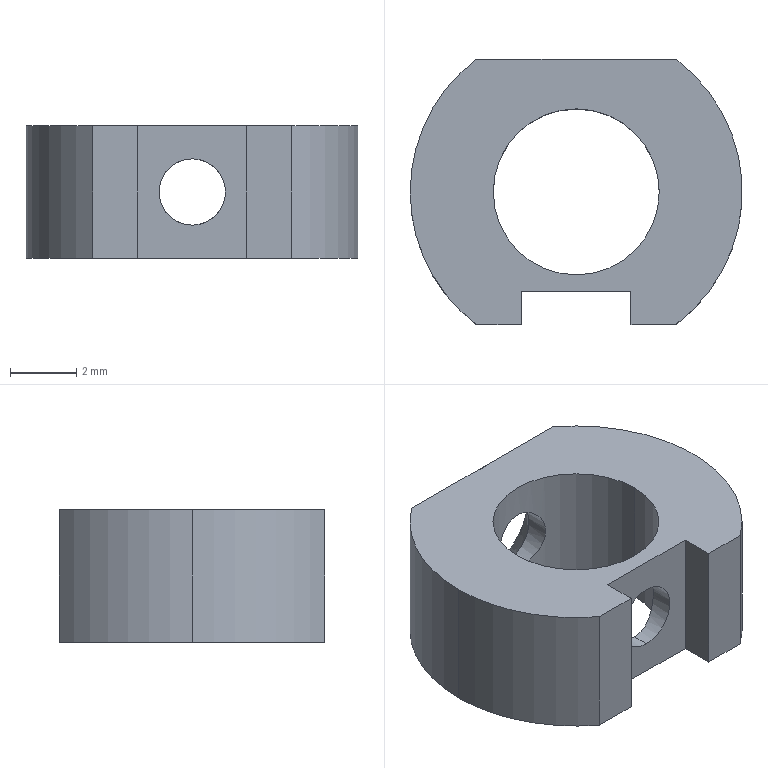Part | SolidWorks | features BaseBody 1 | 1 solid | 20 faces | box 10 x 8 x 4 mm | volume 178.926 mm3 | cylinder 9 | plane 9 | cone 2 | commonest cylinder face diameters 2 x4 10 x3 5 x2
STEP:
#1=CARTESIAN_POINT('',(-5.,0.,4.5));
#2=VERTEX_POINT('',#1);
#3=CARTESIAN_POINT('',(-3.,-4.,4.5));
#4=VERTEX_POINT('',#3);
#5=CARTESIAN_POINT('',(0.,0.,4.5));
#6=DIRECTION('',(0.,0.,1.));
#7=DIRECTION('',(-1.,0.,0.));
#8=AXIS2_PLACEMENT_3D('',#5,#6,#7);
#9=CIRCLE('',#8,5.);
#10=EDGE_CURVE('',#2,#4,#9,.T.);
#11=ORIENTED_EDGE('',*,*,#10,.F.);
#12=CARTESIAN_POINT('',(-5.,0.,0.5));
#13=VERTEX_POINT('',#12);
#14=CARTESIAN_POINT('',(-5.,0.,5.));
#15=DIRECTION('',(0.,0.,-1.));
#16=VECTOR('',#15,1000.);
#17=LINE('',#14,#16);
#18=EDGE_CURVE('',#2,#13,#17,.T.);
#19=ORIENTED_EDGE('',*,*,#18,.T.);
#20=CARTESIAN_POINT('',(-3.,-4.,0.5));
#21=VERTEX_POINT('',#20);
#22=CARTESIAN_POINT('',(0.,0.,0.5));
#23=DIRECTION('',(0.,0.,1.));
#24=DIRECTION('',(-1.,0.,0.));
#25=AXIS2_PLACEMENT_3D('',#22,#23,#24);
#26=CIRCLE('',#25,5.);
#27=EDGE_CURVE('',#13,#21,#26,.T.);
#28=ORIENTED_EDGE('',*,*,#27,.T.);
#29=CARTESIAN_POINT('',(-3.,-4.,5.));
#30=DIRECTION('',(0.,0.,1.));
#31=VECTOR('',#30,1000.);
#32=LINE('',#29,#31);
#33=EDGE_CURVE('',#21,#4,#32,.T.);
#34=ORIENTED_EDGE('',*,*,#33,.T.);
#35=EDGE_LOOP('',(#11,#19,#28,#34));
#36=FACE_OUTER_BOUND('',#35,.T.);
#37=CARTESIAN_POINT('',(0.,0.,5.));
#38=DIRECTION('',(0.,0.,-1.));
#39=DIRECTION('',(-1.,0.,0.));
#40=AXIS2_PLACEMENT_3D('',#37,#38,#39);
#41=CYLINDRICAL_SURFACE('',#40,5.);
#42=ADVANCED_FACE('',(#36),#41,.T.);
#43=CARTESIAN_POINT('',(0.,-2.5,3.5));
#44=VERTEX_POINT('',#43);
#45=CARTESIAN_POINT('',(0.,-2.5,1.5));
#46=VERTEX_POINT('',#45);
#47=CARTESIAN_POINT('',(0.,-2.5,3.5));
#48=CARTESIAN_POINT('',(0.1336,-2.5,3.5));
#49=CARTESIAN_POINT('',(0.2646,-2.489,3.473));
#50=CARTESIAN_POINT('',(0.5062,-2.451,3.372));
#51=CARTESIAN_POINT('',(0.6161,-2.425,3.298));
#52=CARTESIAN_POINT('',(0.7985,-2.371,3.116));
#53=CARTESIAN_POINT('',(0.8726,-2.343,3.006));
#54=CARTESIAN_POINT('',(0.9728,-2.304,2.766));
#55=CARTESIAN_POINT('',(0.9998,-2.291,2.633));
#56=CARTESIAN_POINT('',(1.,-2.291,2.369));
#57=CARTESIAN_POINT('',(0.9739,-2.303,2.238));
#58=CARTESIAN_POINT('',(0.8725,-2.343,1.994));
#59=CARTESIAN_POINT('',(0.799,-2.371,1.885));
#60=CARTESIAN_POINT('',(0.6162,-2.425,1.702));
#61=CARTESIAN_POINT('',(0.506,-2.451,1.628));
#62=CARTESIAN_POINT('',(0.2658,-2.489,1.527));
#63=CARTESIAN_POINT('',(0.1336,-2.5,1.5));
#64=CARTESIAN_POINT('',(0.,-2.5,1.5));
#65=B_SPLINE_CURVE_WITH_KNOTS('',3,(#47,#48,#49,#50,#51,#52,#53,#54,#55,#56,#57,#58,#59,#60,#61,#62,#63,#64),.UNSPECIFIED.,.F.,.F.,(4,2,2,2,2,2,2,2,4),(0.,0.0003948,0.0007896,0.001184,0.001579,0.001974,0.002369,0.002764,0.003158),.UNSPECIFIED.);
#66=EDGE_CURVE('',#44,#46,#65,.T.);
#67=ORIENTED_EDGE('',*,*,#66,.F.);
#68=CARTESIAN_POINT('',(0.,-2.5,1.5));
#69=CARTESIAN_POINT('',(-0.1336,-2.5,1.5));
#70=CARTESIAN_POINT('',(-0.2646,-2.489,1.527));
#71=CARTESIAN_POINT('',(-0.5062,-2.451,1.628));
#72=CARTESIAN_POINT('',(-0.6161,-2.425,1.702));
#73=CARTESIAN_POINT('',(-0.7985,-2.371,1.884));
#74=CARTESIAN_POINT('',(-0.8726,-2.343,1.994));
#75=CARTESIAN_POINT('',(-0.9728,-2.304,2.234));
#76=CARTESIAN_POINT('',(-0.9998,-2.291,2.367));
#77=CARTESIAN_POINT('',(-1.,-2.291,2.631));
#78=CARTESIAN_POINT('',(-0.9739,-2.303,2.762));
#79=CARTESIAN_POINT('',(-0.8725,-2.343,3.006));
#80=CARTESIAN_POINT('',(-0.799,-2.371,3.115));
#81=CARTESIAN_POINT('',(-0.6162,-2.425,3.298));
#82=CARTESIAN_POINT('',(-0.506,-2.451,3.372));
#83=CARTESIAN_POINT('',(-0.2658,-2.489,3.473));
#84=CARTESIAN_POINT('',(-0.1336,-2.5,3.5));
#85=CARTESIAN_POINT('',(0.,-2.5,3.5));
#86=B_SPLINE_CURVE_WITH_KNOTS('',3,(#68,#69,#70,#71,#72,#73,#74,#75,#76,#77,#78,#79,#80,#81,#82,#83,#84,#85),.UNSPECIFIED.,.F.,.F.,(4,2,2,2,2,2,2,2,4),(0.003158,0.003553,0.003948,0.004343,0.004737,0.005132,0.005527,0.005921,0.006316),.UNSPECIFIED.);
#87=EDGE_CURVE('',#46,#44,#86,.T.);
#88=ORIENTED_EDGE('',*,*,#87,.F.);
#89=EDGE_LOOP('',(#67,#88));
#90=FACE_BOUND('',#89,.T.);
#91=CARTESIAN_POINT('',(2.5,0.,4.5));
#92=VERTEX_POINT('',#91);
#93=CARTESIAN_POINT('',(-2.5,0.,4.5));
#94=VERTEX_POINT('',#93);
#95=CARTESIAN_POINT('',(0.,0.,4.5));
#96=DIRECTION('',(0.,0.,-1.));
#97=DIRECTION('',(-1.,0.,0.));
#98=AXIS2_PLACEMENT_3D('',#95,#96,#97);
#99=CIRCLE('',#98,2.5);
#100=EDGE_CURVE('',#92,#94,#99,.T.);
#101=ORIENTED_EDGE('',*,*,#100,.F.);
#102=CARTESIAN_POINT('',(2.5,0.,0.5));
#103=VERTEX_POINT('',#102);
#104=CARTESIAN_POINT('',(2.5,0.,5.));
#105=DIRECTION('',(0.,0.,-1.));
#106=VECTOR('',#105,1000.);
#107=LINE('',#104,#106);
#108=EDGE_CURVE('',#92,#103,#107,.T.);
#109=ORIENTED_EDGE('',*,*,#108,.T.);
#110=CARTESIAN_POINT('',(-2.5,0.,0.5));
#111=VERTEX_POINT('',#110);
#112=CARTESIAN_POINT('',(0.,0.,0.5));
#113=DIRECTION('',(0.,0.,1.));
#114=DIRECTION('',(-1.,0.,0.));
#115=AXIS2_PLACEMENT_3D('',#112,#113,#114);
#116=CIRCLE('',#115,2.5);
#117=EDGE_CURVE('',#111,#103,#116,.T.);
#118=ORIENTED_EDGE('',*,*,#117,.F.);
#119=CARTESIAN_POINT('',(-2.5,0.,5.));
#120=DIRECTION('',(0.,0.,-1.));
#121=VECTOR('',#120,1000.);
#122=LINE('',#119,#121);
#123=EDGE_CURVE('',#94,#111,#122,.T.);
#124=ORIENTED_EDGE('',*,*,#123,.F.);
#125=EDGE_LOOP('',(#101,#109,#118,#124));
#126=FACE_OUTER_BOUND('',#125,.T.);
#127=CARTESIAN_POINT('',(0.,0.,5.));
#128=DIRECTION('',(0.,0.,-1.));
#129=DIRECTION('',(-1.,0.,0.));
#130=AXIS2_PLACEMENT_3D('',#127,#128,#129);
#131=CYLINDRICAL_SURFACE('',#130,2.5);
#132=ADVANCED_FACE('',(#90,#126),#131,.F.);
#133=CARTESIAN_POINT('',(0.,-3.,3.5));
#134=VERTEX_POINT('',#133);
#135=CARTESIAN_POINT('',(0.,-3.,1.5));
#136=VERTEX_POINT('',#135);
#137=CARTESIAN_POINT('',(0.,-3.,2.5));
#138=DIRECTION('',(0.,-1.,0.));
#139=DIRECTION('',(0.,0.,1.));
#140=AXIS2_PLACEMENT_3D('',#137,#138,#139);
#141=CIRCLE('',#140,1.);
#142=EDGE_CURVE('',#134,#136,#141,.T.);
#143=ORIENTED_EDGE('',*,*,#142,.T.);
#144=CARTESIAN_POINT('',(0.,-6.,1.5));
#145=DIRECTION('',(0.,1.,0.));
#146=VECTOR('',#145,1000.);
#147=LINE('',#144,#146);
#148=EDGE_CURVE('',#136,#46,#147,.T.);
#149=ORIENTED_EDGE('',*,*,#148,.T.);
#150=ORIENTED_EDGE('',*,*,#87,.T.);
#151=CARTESIAN_POINT('',(0.,-6.,3.5));
#152=DIRECTION('',(0.,1.,0.));
#153=VECTOR('',#152,1000.);
#154=LINE('',#151,#153);
#155=EDGE_CURVE('',#134,#44,#154,.T.);
#156=ORIENTED_EDGE('',*,*,#155,.F.);
#157=EDGE_LOOP('',(#143,#149,#150,#156));
#158=FACE_OUTER_BOUND('',#157,.T.);
#159=CARTESIAN_POINT('',(0.,-6.,2.5));
#160=DIRECTION('',(0.,1.,0.));
#161=DIRECTION('',(0.,0.,1.));
#162=AXIS2_PLACEMENT_3D('',#159,#160,#161);
#163=CYLINDRICAL_SURFACE('',#162,1.);
#164=ADVANCED_FACE('',(#158),#163,.F.);
#165=CARTESIAN_POINT('',(0.,3.,1.5));
#166=VERTEX_POINT('',#165);
#167=CARTESIAN_POINT('',(0.,3.,3.5));
#168=VERTEX_POINT('',#167);
#169=CARTESIAN_POINT('',(0.,3.,2.5));
#170=DIRECTION('',(0.,1.,0.));
#171=DIRECTION('',(0.,0.,1.));
#172=AXIS2_PLACEMENT_3D('',#169,#170,#171);
#173=CIRCLE('',#172,1.);
#174=EDGE_CURVE('',#166,#168,#173,.T.);
#175=ORIENTED_EDGE('',*,*,#174,.F.);
#176=CARTESIAN_POINT('',(0.,4.,0.5));
#177=VERTEX_POINT('',#176);
#178=CARTESIAN_POINT('',(0.,4.,0.5));
#179=DIRECTION('',(0.,0.7071,-0.7071));
#180=VECTOR('',#179,1000.);
#181=LINE('',#178,#180);
#182=EDGE_CURVE('',#166,#177,#181,.T.);
#183=ORIENTED_EDGE('',*,*,#182,.T.);
#184=CARTESIAN_POINT('',(0.,4.,4.5));
#185=VERTEX_POINT('',#184);
#186=CARTESIAN_POINT('',(0.,4.,2.5));
#187=DIRECTION('',(0.,1.,0.));
#188=DIRECTION('',(0.,0.,1.));
#189=AXIS2_PLACEMENT_3D('',#186,#187,#188);
#190=CIRCLE('',#189,2.);
#191=EDGE_CURVE('',#177,#185,#190,.T.);
#192=ORIENTED_EDGE('',*,*,#191,.T.);
#193=CARTESIAN_POINT('',(0.,4.,4.5));
#194=DIRECTION('',(0.,0.7071,0.7071));
#195=VECTOR('',#194,1000.);
#196=LINE('',#193,#195);
#197=EDGE_CURVE('',#168,#185,#196,.T.);
#198=ORIENTED_EDGE('',*,*,#197,.F.);
#199=EDGE_LOOP('',(#175,#183,#192,#198));
#200=FACE_OUTER_BOUND('',#199,.T.);
#201=CARTESIAN_POINT('',(0.,4.,2.5));
#202=DIRECTION('',(0.,1.,0.));
#203=DIRECTION('',(0.,0.,1.));
#204=AXIS2_PLACEMENT_3D('',#201,#202,#203);
#205=CONICAL_SURFACE('',#204,2.,0.7854);
#206=ADVANCED_FACE('',(#200),#205,.F.);
#207=CARTESIAN_POINT('',(0.,2.5,3.5));
#208=VERTEX_POINT('',#207);
#209=CARTESIAN_POINT('',(0.,2.5,1.5));
#210=VERTEX_POINT('',#209);
#211=CARTESIAN_POINT('',(0.,2.5,3.5));
#212=CARTESIAN_POINT('',(-0.1336,2.5,3.5));
#213=CARTESIAN_POINT('',(-0.2646,2.489,3.473));
#214=CARTESIAN_POINT('',(-0.5062,2.451,3.372));
#215=CARTESIAN_POINT('',(-0.6161,2.425,3.298));
#216=CARTESIAN_POINT('',(-0.7985,2.371,3.116));
#217=CARTESIAN_POINT('',(-0.8726,2.343,3.006));
#218=CARTESIAN_POINT('',(-0.9728,2.304,2.766));
#219=CARTESIAN_POINT('',(-0.9998,2.291,2.633));
#220=CARTESIAN_POINT('',(-1.,2.291,2.369));
#221=CARTESIAN_POINT('',(-0.9739,2.303,2.238));
#222=CARTESIAN_POINT('',(-0.8725,2.343,1.994));
#223=CARTESIAN_POINT('',(-0.799,2.371,1.885));
#224=CARTESIAN_POINT('',(-0.6162,2.425,1.702));
#225=CARTESIAN_POINT('',(-0.506,2.451,1.628));
#226=CARTESIAN_POINT('',(-0.2658,2.489,1.527));
#227=CARTESIAN_POINT('',(-0.1336,2.5,1.5));
#228=CARTESIAN_POINT('',(0.,2.5,1.5));
#229=B_SPLINE_CURVE_WITH_KNOTS('',3,(#211,#212,#213,#214,#215,#216,#217,#218,#219,#220,#221,#222,#223,#224,#225,#226,#227,#228),.UNSPECIFIED.,.F.,.F.,(4,2,2,2,2,2,2,2,4),(0.,0.0003948,0.0007896,0.001184,0.001579,0.001974,0.002369,0.002764,0.003158),.UNSPECIFIED.);
#230=EDGE_CURVE('',#208,#210,#229,.T.);
#231=ORIENTED_EDGE('',*,*,#230,.T.);
#232=CARTESIAN_POINT('',(0.,-6.,1.5));
#233=DIRECTION('',(0.,1.,0.));
#234=VECTOR('',#233,1000.);
#235=LINE('',#232,#234);
#236=EDGE_CURVE('',#210,#166,#235,.T.);
#237=ORIENTED_EDGE('',*,*,#236,.T.);
#238=ORIENTED_EDGE('',*,*,#174,.T.);
#239=CARTESIAN_POINT('',(0.,-6.,3.5));
#240=DIRECTION('',(0.,1.,0.));
#241=VECTOR('',#240,1000.);
#242=LINE('',#239,#241);
#243=EDGE_CURVE('',#208,#168,#242,.T.);
#244=ORIENTED_EDGE('',*,*,#243,.F.);
#245=EDGE_LOOP('',(#231,#237,#238,#244));
#246=FACE_OUTER_BOUND('',#245,.T.);
#247=CARTESIAN_POINT('',(0.,-6.,2.5));
#248=DIRECTION('',(0.,1.,0.));
#249=DIRECTION('',(0.,0.,1.));
#250=AXIS2_PLACEMENT_3D('',#247,#248,#249);
#251=CYLINDRICAL_SURFACE('',#250,1.);
#252=ADVANCED_FACE('',(#246),#251,.F.);
#253=CARTESIAN_POINT('',(-1.65,-3.,4.5));
#254=VERTEX_POINT('',#253);
#255=CARTESIAN_POINT('',(1.65,-3.,4.5));
#256=VERTEX_POINT('',#255);
#257=CARTESIAN_POINT('',(0.,-3.,4.5));
#258=DIRECTION('',(1.,0.,0.));
#259=VECTOR('',#258,1000.);
#260=LINE('',#257,#259);
#261=EDGE_CURVE('',#254,#256,#260,.T.);
#262=ORIENTED_EDGE('',*,*,#261,.T.);
#263=CARTESIAN_POINT('',(1.65,-4.,4.5));
#264=VERTEX_POINT('',#263);
#265=CARTESIAN_POINT('',(1.65,-3.,4.5));
#266=DIRECTION('',(0.,-1.,0.));
#267=VECTOR('',#266,1000.);
#268=LINE('',#265,#267);
#269=EDGE_CURVE('',#256,#264,#268,.T.);
#270=ORIENTED_EDGE('',*,*,#269,.T.);
#271=CARTESIAN_POINT('',(3.,-4.,4.5));
#272=VERTEX_POINT('',#271);
#273=CARTESIAN_POINT('',(6.418,-4.,4.5));
#274=DIRECTION('',(1.,0.,0.));
#275=VECTOR('',#274,1000.);
#276=LINE('',#273,#275);
#277=EDGE_CURVE('',#264,#272,#276,.T.);
#278=ORIENTED_EDGE('',*,*,#277,.T.);
#279=CARTESIAN_POINT('',(3.,4.,4.5));
#280=VERTEX_POINT('',#279);
#281=CARTESIAN_POINT('',(0.,0.,4.5));
#282=DIRECTION('',(0.,0.,1.));
#283=DIRECTION('',(-1.,0.,0.));
#284=AXIS2_PLACEMENT_3D('',#281,#282,#283);
#285=CIRCLE('',#284,5.);
#286=EDGE_CURVE('',#272,#280,#285,.T.);
#287=ORIENTED_EDGE('',*,*,#286,.T.);
#288=CARTESIAN_POINT('',(0.,4.,4.5));
#289=DIRECTION('',(-1.,0.,0.));
#290=VECTOR('',#289,1000.);
#291=LINE('',#288,#290);
#292=EDGE_CURVE('',#280,#185,#291,.T.);
#293=ORIENTED_EDGE('',*,*,#292,.T.);
#294=CARTESIAN_POINT('',(-3.,4.,4.5));
#295=VERTEX_POINT('',#294);
#296=CARTESIAN_POINT('',(0.,4.,4.5));
#297=DIRECTION('',(-1.,0.,0.));
#298=VECTOR('',#297,1000.);
#299=LINE('',#296,#298);
#300=EDGE_CURVE('',#185,#295,#299,.T.);
#301=ORIENTED_EDGE('',*,*,#300,.T.);
#302=CARTESIAN_POINT('',(0.,0.,4.5));
#303=DIRECTION('',(0.,0.,1.));
#304=DIRECTION('',(-1.,0.,0.));
#305=AXIS2_PLACEMENT_3D('',#302,#303,#304);
#306=CIRCLE('',#305,5.);
#307=EDGE_CURVE('',#295,#2,#306,.T.);
#308=ORIENTED_EDGE('',*,*,#307,.T.);
#309=ORIENTED_EDGE('',*,*,#10,.T.);
#310=CARTESIAN_POINT('',(-1.65,-4.,4.5));
#311=VERTEX_POINT('',#310);
#312=CARTESIAN_POINT('',(6.418,-4.,4.5));
#313=DIRECTION('',(1.,0.,0.));
#314=VECTOR('',#313,1000.);
#315=LINE('',#312,#314);
#316=EDGE_CURVE('',#4,#311,#315,.T.);
#317=ORIENTED_EDGE('',*,*,#316,.T.);
#318=CARTESIAN_POINT('',(-1.65,-3.,4.5));
#319=DIRECTION('',(0.,1.,0.));
#320=VECTOR('',#319,1000.);
#321=LINE('',#318,#320);
#322=EDGE_CURVE('',#311,#254,#321,.T.);
#323=ORIENTED_EDGE('',*,*,#322,.T.);
#324=EDGE_LOOP('',(#262,#270,#278,#287,#293,#301,#308,#309,#317,#323));
#325=FACE_OUTER_BOUND('',#324,.T.);
#326=CARTESIAN_POINT('',(0.,0.,4.5));
#327=DIRECTION('',(0.,0.,-1.));
#328=DIRECTION('',(-1.,0.,0.));
#329=AXIS2_PLACEMENT_3D('',#326,#327,#328);
#330=CIRCLE('',#329,2.5);
#331=EDGE_CURVE('',#94,#92,#330,.T.);
#332=ORIENTED_EDGE('',*,*,#331,.T.);
#333=ORIENTED_EDGE('',*,*,#100,.T.);
#334=EDGE_LOOP('',(#332,#333));
#335=FACE_BOUND('',#334,.T.);
#336=CARTESIAN_POINT('',(0.,0.,4.5));
#337=DIRECTION('',(0.,0.,1.));
#338=DIRECTION('',(1.,0.,0.));
#339=AXIS2_PLACEMENT_3D('',#336,#337,#338);
#340=PLANE('',#339);
#341=ADVANCED_FACE('',(#325,#335),#340,.T.);
#342=CARTESIAN_POINT('',(1.65,-3.,0.5));
#343=VERTEX_POINT('',#342);
#344=CARTESIAN_POINT('',(1.65,-3.,0.));
#345=DIRECTION('',(0.,0.,-1.));
#346=VECTOR('',#345,1000.);
#347=LINE('',#344,#346);
#348=EDGE_CURVE('',#256,#343,#347,.T.);
#349=ORIENTED_EDGE('',*,*,#348,.F.);
#350=ORIENTED_EDGE('',*,*,#261,.F.);
#351=CARTESIAN_POINT('',(-1.65,-3.,0.5));
#352=VERTEX_POINT('',#351);
#353=CARTESIAN_POINT('',(-1.65,-3.,0.));
#354=DIRECTION('',(0.,0.,1.));
#355=VECTOR('',#354,1000.);
#356=LINE('',#353,#355);
#357=EDGE_CURVE('',#352,#254,#356,.T.);
#358=ORIENTED_EDGE('',*,*,#357,.F.);
#359=CARTESIAN_POINT('',(0.,-3.,0.5));
#360=DIRECTION('',(-1.,0.,0.));
#361=VECTOR('',#360,1000.);
#362=LINE('',#359,#361);
#363=EDGE_CURVE('',#343,#352,#362,.T.);
#364=ORIENTED_EDGE('',*,*,#363,.F.);
#365=EDGE_LOOP('',(#349,#350,#358,#364));
#366=FACE_OUTER_BOUND('',#365,.T.);
#367=ORIENTED_EDGE('',*,*,#142,.F.);
#368=CARTESIAN_POINT('',(0.,-3.,2.5));
#369=DIRECTION('',(0.,-1.,0.));
#370=DIRECTION('',(0.,0.,1.));
#371=AXIS2_PLACEMENT_3D('',#368,#369,#370);
#372=CIRCLE('',#371,1.);
#373=EDGE_CURVE('',#136,#134,#372,.T.);
#374=ORIENTED_EDGE('',*,*,#373,.F.);
#375=EDGE_LOOP('',(#367,#374));
#376=FACE_BOUND('',#375,.T.);
#377=CARTESIAN_POINT('',(0.,-3.,0.));
#378=DIRECTION('',(0.,1.,0.));
#379=DIRECTION('',(0.,0.,1.));
#380=AXIS2_PLACEMENT_3D('',#377,#378,#379);
#381=PLANE('',#380);
#382=ADVANCED_FACE('',(#366,#376),#381,.F.);
#383=ORIENTED_EDGE('',*,*,#18,.F.);
#384=ORIENTED_EDGE('',*,*,#307,.F.);
#385=CARTESIAN_POINT('',(-3.,4.,0.5));
#386=VERTEX_POINT('',#385);
#387=CARTESIAN_POINT('',(-3.,4.,5.));
#388=DIRECTION('',(0.,0.,-1.));
#389=VECTOR('',#388,1000.);
#390=LINE('',#387,#389);
#391=EDGE_CURVE('',#295,#386,#390,.T.);
#392=ORIENTED_EDGE('',*,*,#391,.T.);
#393=CARTESIAN_POINT('',(0.,0.,0.5));
#394=DIRECTION('',(0.,0.,1.));
#395=DIRECTION('',(-1.,0.,0.));
#396=AXIS2_PLACEMENT_3D('',#393,#394,#395);
#397=CIRCLE('',#396,5.);
#398=EDGE_CURVE('',#386,#13,#397,.T.);
#399=ORIENTED_EDGE('',*,*,#398,.T.);
#400=EDGE_LOOP('',(#383,#384,#392,#399));
#401=FACE_OUTER_BOUND('',#400,.T.);
#402=CARTESIAN_POINT('',(0.,0.,5.));
#403=DIRECTION('',(0.,0.,-1.));
#404=DIRECTION('',(-1.,0.,0.));
#405=AXIS2_PLACEMENT_3D('',#402,#403,#404);
#406=CYLINDRICAL_SURFACE('',#405,5.);
#407=ADVANCED_FACE('',(#401),#406,.T.);
#408=ORIENTED_EDGE('',*,*,#391,.F.);
#409=ORIENTED_EDGE('',*,*,#300,.F.);
#410=ORIENTED_EDGE('',*,*,#191,.F.);
#411=CARTESIAN_POINT('',(6.418,4.,0.5));
#412=DIRECTION('',(1.,0.,0.));
#413=VECTOR('',#412,1000.);
#414=LINE('',#411,#413);
#415=EDGE_CURVE('',#386,#177,#414,.T.);
#416=ORIENTED_EDGE('',*,*,#415,.F.);
#417=EDGE_LOOP('',(#408,#409,#410,#416));
#418=FACE_OUTER_BOUND('',#417,.T.);
#419=CARTESIAN_POINT('',(6.418,4.,5.));
#420=DIRECTION('',(0.,-1.,0.));
#421=DIRECTION('',(0.,0.,-1.));
#422=AXIS2_PLACEMENT_3D('',#419,#420,#421);
#423=PLANE('',#422);
#424=ADVANCED_FACE('',(#418),#423,.F.);
#425=CARTESIAN_POINT('',(0.,4.,2.5));
#426=DIRECTION('',(0.,1.,0.));
#427=DIRECTION('',(0.,0.,1.));
#428=AXIS2_PLACEMENT_3D('',#425,#426,#427);
#429=CIRCLE('',#428,2.);
#430=EDGE_CURVE('',#185,#177,#429,.T.);
#431=ORIENTED_EDGE('',*,*,#430,.F.);
#432=ORIENTED_EDGE('',*,*,#292,.F.);
#433=CARTESIAN_POINT('',(3.,4.,0.5));
#434=VERTEX_POINT('',#433);
#435=CARTESIAN_POINT('',(3.,4.,5.));
#436=DIRECTION('',(0.,0.,1.));
#437=VECTOR('',#436,1000.);
#438=LINE('',#435,#437);
#439=EDGE_CURVE('',#434,#280,#438,.T.);
#440=ORIENTED_EDGE('',*,*,#439,.F.);
#441=CARTESIAN_POINT('',(6.418,4.,0.5));
#442=DIRECTION('',(1.,0.,0.));
#443=VECTOR('',#442,1000.);
#444=LINE('',#441,#443);
#445=EDGE_CURVE('',#177,#434,#444,.T.);
#446=ORIENTED_EDGE('',*,*,#445,.F.);
#447=EDGE_LOOP('',(#431,#432,#440,#446));
#448=FACE_OUTER_BOUND('',#447,.T.);
#449=CARTESIAN_POINT('',(6.418,4.,5.));
#450=DIRECTION('',(0.,-1.,0.));
#451=DIRECTION('',(0.,0.,-1.));
#452=AXIS2_PLACEMENT_3D('',#449,#450,#451);
#453=PLANE('',#452);
#454=ADVANCED_FACE('',(#448),#453,.F.);
#455=ORIENTED_EDGE('',*,*,#286,.F.);
#456=CARTESIAN_POINT('',(3.,-4.,0.5));
#457=VERTEX_POINT('',#456);
#458=CARTESIAN_POINT('',(3.,-4.,5.));
#459=DIRECTION('',(0.,0.,-1.));
#460=VECTOR('',#459,1000.);
#461=LINE('',#458,#460);
#462=EDGE_CURVE('',#272,#457,#461,.T.);
#463=ORIENTED_EDGE('',*,*,#462,.T.);
#464=CARTESIAN_POINT('',(0.,0.,0.5));
#465=DIRECTION('',(0.,0.,1.));
#466=DIRECTION('',(-1.,0.,0.));
#467=AXIS2_PLACEMENT_3D('',#464,#465,#466);
#468=CIRCLE('',#467,5.);
#469=EDGE_CURVE('',#457,#434,#468,.T.);
#470=ORIENTED_EDGE('',*,*,#469,.T.);
#471=ORIENTED_EDGE('',*,*,#439,.T.);
#472=EDGE_LOOP('',(#455,#463,#470,#471));
#473=FACE_OUTER_BOUND('',#472,.T.);
#474=CARTESIAN_POINT('',(0.,0.,5.));
#475=DIRECTION('',(0.,0.,-1.));
#476=DIRECTION('',(-1.,0.,0.));
#477=AXIS2_PLACEMENT_3D('',#474,#475,#476);
#478=CYLINDRICAL_SURFACE('',#477,5.);
#479=ADVANCED_FACE('',(#473),#478,.T.);
#480=ORIENTED_EDGE('',*,*,#108,.F.);
#481=ORIENTED_EDGE('',*,*,#331,.F.);
#482=ORIENTED_EDGE('',*,*,#123,.T.);
#483=CARTESIAN_POINT('',(0.,0.,0.5));
#484=DIRECTION('',(0.,0.,1.));
#485=DIRECTION('',(-1.,0.,0.));
#486=AXIS2_PLACEMENT_3D('',#483,#484,#485);
#487=CIRCLE('',#486,2.5);
#488=EDGE_CURVE('',#103,#111,#487,.T.);
#489=ORIENTED_EDGE('',*,*,#488,.F.);
#490=EDGE_LOOP('',(#480,#481,#482,#489));
#491=FACE_OUTER_BOUND('',#490,.T.);
#492=ORIENTED_EDGE('',*,*,#230,.F.);
#493=CARTESIAN_POINT('',(0.,2.5,1.5));
#494=CARTESIAN_POINT('',(0.1336,2.5,1.5));
#495=CARTESIAN_POINT('',(0.2646,2.489,1.527));
#496=CARTESIAN_POINT('',(0.5062,2.451,1.628));
#497=CARTESIAN_POINT('',(0.6161,2.425,1.702));
#498=CARTESIAN_POINT('',(0.7985,2.371,1.884));
#499=CARTESIAN_POINT('',(0.8726,2.343,1.994));
#500=CARTESIAN_POINT('',(0.9728,2.304,2.234));
#501=CARTESIAN_POINT('',(0.9998,2.291,2.367));
#502=CARTESIAN_POINT('',(1.,2.291,2.631));
#503=CARTESIAN_POINT('',(0.9739,2.303,2.762));
#504=CARTESIAN_POINT('',(0.8725,2.343,3.006));
#505=CARTESIAN_POINT('',(0.799,2.371,3.115));
#506=CARTESIAN_POINT('',(0.6162,2.425,3.298));
#507=CARTESIAN_POINT('',(0.506,2.451,3.372));
#508=CARTESIAN_POINT('',(0.2658,2.489,3.473));
#509=CARTESIAN_POINT('',(0.1336,2.5,3.5));
#510=CARTESIAN_POINT('',(0.,2.5,3.5));
#511=B_SPLINE_CURVE_WITH_KNOTS('',3,(#493,#494,#495,#496,#497,#498,#499,#500,#501,#502,#503,#504,#505,#506,#507,#508,#509,#510),.UNSPECIFIED.,.F.,.F.,(4,2,2,2,2,2,2,2,4),(0.003158,0.003553,0.003948,0.004343,0.004737,0.005132,0.005527,0.005921,0.006316),.UNSPECIFIED.);
#512=EDGE_CURVE('',#210,#208,#511,.T.);
#513=ORIENTED_EDGE('',*,*,#512,.F.);
#514=EDGE_LOOP('',(#492,#513));
#515=FACE_BOUND('',#514,.T.);
#516=CARTESIAN_POINT('',(0.,0.,5.));
#517=DIRECTION('',(0.,0.,-1.));
#518=DIRECTION('',(-1.,0.,0.));
#519=AXIS2_PLACEMENT_3D('',#516,#517,#518);
#520=CYLINDRICAL_SURFACE('',#519,2.5);
#521=ADVANCED_FACE('',(#491,#515),#520,.F.);
#522=ORIENTED_EDGE('',*,*,#415,.T.);
#523=ORIENTED_EDGE('',*,*,#445,.T.);
#524=ORIENTED_EDGE('',*,*,#469,.F.);
#525=CARTESIAN_POINT('',(1.65,-4.,0.5));
#526=VERTEX_POINT('',#525);
#527=CARTESIAN_POINT('',(0.,-4.,0.5));
#528=DIRECTION('',(-1.,0.,0.));
#529=VECTOR('',#528,1000.);
#530=LINE('',#527,#529);
#531=EDGE_CURVE('',#457,#526,#530,.T.);
#532=ORIENTED_EDGE('',*,*,#531,.T.);
#533=CARTESIAN_POINT('',(1.65,0.,0.5));
#534=DIRECTION('',(0.,1.,0.));
#535=VECTOR('',#534,1000.);
#536=LINE('',#533,#535);
#537=EDGE_CURVE('',#526,#343,#536,.T.);
#538=ORIENTED_EDGE('',*,*,#537,.T.);
#539=ORIENTED_EDGE('',*,*,#363,.T.);
#540=CARTESIAN_POINT('',(-1.65,-4.,0.5));
#541=VERTEX_POINT('',#540);
#542=CARTESIAN_POINT('',(-1.65,0.,0.5));
#543=DIRECTION('',(0.,-1.,0.));
#544=VECTOR('',#543,1000.);
#545=LINE('',#542,#544);
#546=EDGE_CURVE('',#352,#541,#545,.T.);
#547=ORIENTED_EDGE('',*,*,#546,.T.);
#548=CARTESIAN_POINT('',(0.,-4.,0.5));
#549=DIRECTION('',(-1.,0.,0.));
#550=VECTOR('',#549,1000.);
#551=LINE('',#548,#550);
#552=EDGE_CURVE('',#541,#21,#551,.T.);
#553=ORIENTED_EDGE('',*,*,#552,.T.);
#554=ORIENTED_EDGE('',*,*,#27,.F.);
#555=ORIENTED_EDGE('',*,*,#398,.F.);
#556=EDGE_LOOP('',(#522,#523,#524,#532,#538,#539,#547,#553,#554,#555));
#557=FACE_OUTER_BOUND('',#556,.T.);
#558=ORIENTED_EDGE('',*,*,#117,.T.);
#559=ORIENTED_EDGE('',*,*,#488,.T.);
#560=EDGE_LOOP('',(#558,#559));
#561=FACE_BOUND('',#560,.T.);
#562=CARTESIAN_POINT('',(0.,0.,0.5));
#563=DIRECTION('',(0.,0.,-1.));
#564=DIRECTION('',(-1.,0.,0.));
#565=AXIS2_PLACEMENT_3D('',#562,#563,#564);
#566=PLANE('',#565);
#567=ADVANCED_FACE('',(#557,#561),#566,.T.);
#568=CARTESIAN_POINT('',(1.65,-4.,5.));
#569=DIRECTION('',(0.,0.,-1.));
#570=VECTOR('',#569,1000.);
#571=LINE('',#568,#570);
#572=EDGE_CURVE('',#264,#526,#571,.T.);
#573=ORIENTED_EDGE('',*,*,#572,.F.);
#574=ORIENTED_EDGE('',*,*,#269,.F.);
#575=ORIENTED_EDGE('',*,*,#348,.T.);
#576=ORIENTED_EDGE('',*,*,#537,.F.);
#577=EDGE_LOOP('',(#573,#574,#575,#576));
#578=FACE_OUTER_BOUND('',#577,.T.);
#579=CARTESIAN_POINT('',(1.65,-3.,5.));
#580=DIRECTION('',(1.,0.,0.));
#581=DIRECTION('',(0.,0.,-1.));
#582=AXIS2_PLACEMENT_3D('',#579,#580,#581);
#583=PLANE('',#582);
#584=ADVANCED_FACE('',(#578),#583,.F.);
#585=ORIENTED_EDGE('',*,*,#357,.T.);
#586=ORIENTED_EDGE('',*,*,#322,.F.);
#587=CARTESIAN_POINT('',(-1.65,-4.,0.));
#588=DIRECTION('',(0.,0.,1.));
#589=VECTOR('',#588,1000.);
#590=LINE('',#587,#589);
#591=EDGE_CURVE('',#541,#311,#590,.T.);
#592=ORIENTED_EDGE('',*,*,#591,.F.);
#593=ORIENTED_EDGE('',*,*,#546,.F.);
#594=EDGE_LOOP('',(#585,#586,#592,#593));
#595=FACE_OUTER_BOUND('',#594,.T.);
#596=CARTESIAN_POINT('',(-1.65,-3.,0.));
#597=DIRECTION('',(-1.,0.,0.));
#598=DIRECTION('',(0.,0.,1.));
#599=AXIS2_PLACEMENT_3D('',#596,#597,#598);
#600=PLANE('',#599);
#601=ADVANCED_FACE('',(#595),#600,.F.);
#602=ORIENTED_EDGE('',*,*,#148,.F.);
#603=ORIENTED_EDGE('',*,*,#373,.T.);
#604=ORIENTED_EDGE('',*,*,#155,.T.);
#605=ORIENTED_EDGE('',*,*,#66,.T.);
#606=EDGE_LOOP('',(#602,#603,#604,#605));
#607=FACE_OUTER_BOUND('',#606,.T.);
#608=CARTESIAN_POINT('',(0.,-6.,2.5));
#609=DIRECTION('',(0.,1.,0.));
#610=DIRECTION('',(0.,0.,1.));
#611=AXIS2_PLACEMENT_3D('',#608,#609,#610);
#612=CYLINDRICAL_SURFACE('',#611,1.);
#613=ADVANCED_FACE('',(#607),#612,.F.);
#614=ORIENTED_EDGE('',*,*,#591,.T.);
#615=ORIENTED_EDGE('',*,*,#316,.F.);
#616=ORIENTED_EDGE('',*,*,#33,.F.);
#617=ORIENTED_EDGE('',*,*,#552,.F.);
#618=EDGE_LOOP('',(#614,#615,#616,#617));
#619=FACE_OUTER_BOUND('',#618,.T.);
#620=CARTESIAN_POINT('',(6.418,-4.,5.));
#621=DIRECTION('',(0.,1.,0.));
#622=DIRECTION('',(0.,0.,1.));
#623=AXIS2_PLACEMENT_3D('',#620,#621,#622);
#624=PLANE('',#623);
#625=ADVANCED_FACE('',(#619),#624,.F.);
#626=ORIENTED_EDGE('',*,*,#182,.F.);
#627=CARTESIAN_POINT('',(0.,3.,2.5));
#628=DIRECTION('',(0.,1.,0.));
#629=DIRECTION('',(0.,0.,1.));
#630=AXIS2_PLACEMENT_3D('',#627,#628,#629);
#631=CIRCLE('',#630,1.);
#632=EDGE_CURVE('',#168,#166,#631,.T.);
#633=ORIENTED_EDGE('',*,*,#632,.F.);
#634=ORIENTED_EDGE('',*,*,#197,.T.);
#635=ORIENTED_EDGE('',*,*,#430,.T.);
#636=EDGE_LOOP('',(#626,#633,#634,#635));
#637=FACE_OUTER_BOUND('',#636,.T.);
#638=CARTESIAN_POINT('',(0.,4.,2.5));
#639=DIRECTION('',(0.,1.,0.));
#640=DIRECTION('',(0.,0.,1.));
#641=AXIS2_PLACEMENT_3D('',#638,#639,#640);
#642=CONICAL_SURFACE('',#641,2.,0.7854);
#643=ADVANCED_FACE('',(#637),#642,.F.);
#644=ORIENTED_EDGE('',*,*,#462,.F.);
#645=ORIENTED_EDGE('',*,*,#277,.F.);
#646=ORIENTED_EDGE('',*,*,#572,.T.);
#647=ORIENTED_EDGE('',*,*,#531,.F.);
#648=EDGE_LOOP('',(#644,#645,#646,#647));
#649=FACE_OUTER_BOUND('',#648,.T.);
#650=CARTESIAN_POINT('',(6.418,-4.,5.));
#651=DIRECTION('',(0.,1.,0.));
#652=DIRECTION('',(0.,0.,1.));
#653=AXIS2_PLACEMENT_3D('',#650,#651,#652);
#654=PLANE('',#653);
#655=ADVANCED_FACE('',(#649),#654,.F.);
#656=ORIENTED_EDGE('',*,*,#236,.F.);
#657=ORIENTED_EDGE('',*,*,#512,.T.);
#658=ORIENTED_EDGE('',*,*,#243,.T.);
#659=ORIENTED_EDGE('',*,*,#632,.T.);
#660=EDGE_LOOP('',(#656,#657,#658,#659));
#661=FACE_OUTER_BOUND('',#660,.T.);
#662=CARTESIAN_POINT('',(0.,-6.,2.5));
#663=DIRECTION('',(0.,1.,0.));
#664=DIRECTION('',(0.,0.,1.));
#665=AXIS2_PLACEMENT_3D('',#662,#663,#664);
#666=CYLINDRICAL_SURFACE('',#665,1.);
#667=ADVANCED_FACE('',(#661),#666,.F.);
#668=CLOSED_SHELL('',(#42,#132,#164,#206,#252,#341,#382,#407,#424,#454,#479,#521,#567,#584,#601,#613,#625,#643,#655,#667));
#669=MANIFOLD_SOLID_BREP('',#668);
#670=CARTESIAN_POINT('',(0.,0.,0.));
#671=DIRECTION('',(0.,0.,1.));
#672=DIRECTION('',(1.,0.,0.));
#673=AXIS2_PLACEMENT_3D('',#670,#671,#672);
#674=(LENGTH_UNIT()NAMED_UNIT(*)SI_UNIT(.MILLI.,.METRE.));
#675=UNCERTAINTY_MEASURE_WITH_UNIT(LENGTH_MEASURE(0.00001),#674,'','');
#676=(NAMED_UNIT(*)PLANE_ANGLE_UNIT()SI_UNIT($,.RADIAN.));
#677=(NAMED_UNIT(*)SI_UNIT($,.STERADIAN.)SOLID_ANGLE_UNIT());
#678=(GEOMETRIC_REPRESENTATION_CONTEXT(3)GLOBAL_UNCERTAINTY_ASSIGNED_CONTEXT((#675))GLOBAL_UNIT_ASSIGNED_CONTEXT((#674,#676,#677))REPRESENTATION_CONTEXT('',''));
#679=ADVANCED_BREP_SHAPE_REPRESENTATION('',(#669,#673),#678);